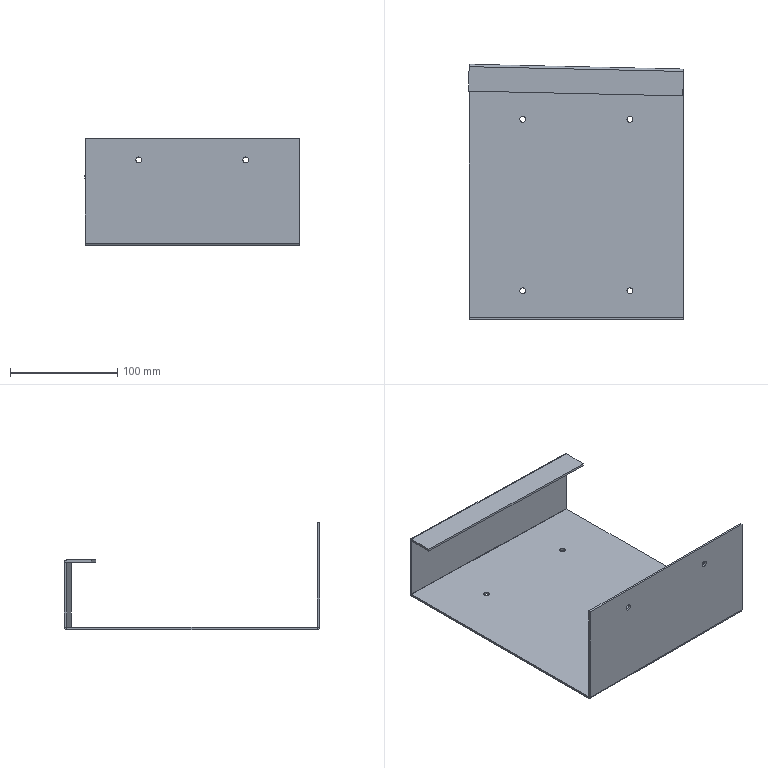Part | STEP file | TS-S54 | 1 solid | 43 faces | box 200.554 x 238.201 x 100 mm | volume 167109 mm3 | plane 24 | cylinder 18 | spline 1 | commonest cylinder face diameters 5.4 x12 0.4 x3 4.4 x3